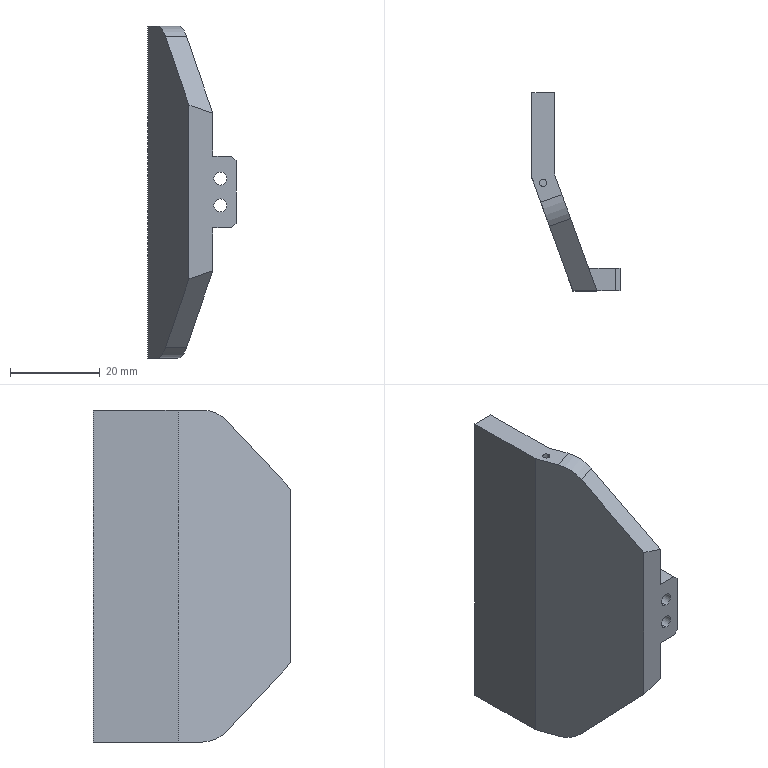NC program | NX | posted with a generic post | part box 19.643 x 44.061 x 74 mm
Lines 1 to 613 of 4832:
N10 G17 G21 G94 G90
(FLOOR_FACING_3 , TOOL : D8开粗)
N12 T02 M6
N14 G54
N16 G17 G0 G90 X44. Y-28.322 B0. C0. S4500 M3
N18 G43 Z29.368 H2
N20 Z2.468
N22 G94 G1 Z-0.532 F800.
N24 X41.
N26 X-41.
N28 Y-24.528
N30 G2 X-40.894 Y-22.939 R12.
N32 G1 X40.894
N34 G3 X38.767 Y-17.557 R12.
N36 G1 X-38.767
N38 G2 X-37.485 Y-16.043 R12.
N40 G1 X-33.616 Y-12.174
N42 X33.616
N44 X28.234 Y-6.792
N46 X-28.234
N48 X-32.477
N50 Z2.468
N52 G0 Z29.368
N54 M5
(FLOOR_FACING_3_COPY , TOOL : D8精光)
N56 T03 M6
N58 G54
N60 G17 G0 G90 X44. Y-28.322 B0. C0. S4500 M3
N62 G43 Z29.368 H3
N64 Z2.368
N66 G94 G1 Z-0.632 F800.
N68 X41.
N70 X-41.
N72 Y-24.528
N74 G2 X-40.894 Y-22.939 R12.
N76 G1 X40.894
N78 G3 X38.767 Y-17.557 R12.
N80 G1 X-38.767
N82 G2 X-37.485 Y-16.043 R12.
N84 G1 X-33.616 Y-12.174
N86 X33.616
N88 X28.234 Y-6.792
N90 X-28.234
N92 X-32.477
N94 Z2.368
N96 G0 Z29.368
N98 M5
(PLANAR_MILL , TOOL : D8开粗)
N100 T02 M6
N102 G54
N104 G17 G0 G90 X-24.188 Y-22.828 B0. C0. S4500 M3
N106 G43 Z29.368 H2
N108 Z0.368
N110 G94 G1 X-26.722 Y-25.362 Z0.363 F2000.
N112 X-26.8 Y-25.55 Z0.362
N114 Y-43.344 Z0.338
N116 X26.8 Z0.263
N118 Y-25.55 Z0.238
N120 X26.722 Y-25.362
N122 X12.775 Y-11.414 Z0.21
N124 X12.481 Y-11.293
N126 X-12.481 Z0.175
N128 X-12.775 Y-11.414 Z0.174
N130 X-26.722 Y-25.362 Z0.147
N132 X-26.8 Y-25.55
N134 Y-43.344 Z0.122
N136 X26.8 Z0.047
N138 Y-25.55 Z0.022
N140 X26.722 Y-25.362
N142 X12.775 Y-11.414 Z-0.006
N144 X12.481 Y-11.293
N146 X-12.481 Z-0.041
N148 X-12.775 Y-11.414 Z-0.042
N150 X-26.722 Y-25.362 Z-0.069
N152 X-26.8 Y-25.55
N154 Y-43.344 Z-0.094
N156 X26.8 Z-0.169
N158 Y-25.55 Z-0.194
N160 X26.722 Y-25.362
N162 X12.775 Y-11.414 Z-0.222
N164 X12.481 Y-11.293
N166 X-12.481 Z-0.257
N168 X-12.775 Y-11.414
N170 X-26.722 Y-25.362 Z-0.285
N172 X-26.8 Y-25.55
N174 Y-43.344 Z-0.31
N176 X26.8 Z-0.385
N178 Y-25.55 Z-0.41
N180 X26.722 Y-25.362
N182 X12.775 Y-11.414 Z-0.438
N184 X12.481 Y-11.293
N186 X-12.481 Z-0.473
N188 X-12.775 Y-11.414
N190 X-26.722 Y-25.362 Z-0.501
N192 X-26.8 Y-25.55
N194 Y-43.344 Z-0.526
N196 X26.8 Z-0.601
N198 Y-25.55 Z-0.626
N200 X26.722 Y-25.362
N202 X12.775 Y-11.414 Z-0.654
N204 X12.481 Y-11.293
N206 X-12.481 Z-0.689
N208 X-12.775 Y-11.414
N210 X-26.722 Y-25.362 Z-0.717
N212 X-26.8 Y-25.55
N214 Y-43.344 Z-0.742
N216 X26.8 Z-0.817
N218 Y-25.55 Z-0.842
N220 X26.722 Y-25.362
N222 X12.775 Y-11.414 Z-0.87
N224 X12.481 Y-11.293
N226 X-12.481 Z-0.905
N228 X-12.775 Y-11.414
N230 X-26.722 Y-25.362 Z-0.933
N232 X-26.8 Y-25.55
N234 Y-43.344 Z-0.958
N236 X26.8 Z-1.033
N238 Y-25.55 Z-1.058
N240 X26.722 Y-25.362
N242 X12.775 Y-11.414 Z-1.085
N244 X12.481 Y-11.293 Z-1.086
N246 X-12.481 Z-1.121
N248 X-12.775 Y-11.414
N250 X-26.722 Y-25.362 Z-1.149
N252 X-26.8 Y-25.55
N254 Y-43.344 Z-1.174
N256 X26.8 Z-1.249
N258 Y-25.55 Z-1.274
N260 X26.722 Y-25.362
N262 X12.775 Y-11.414 Z-1.301
N264 X12.481 Y-11.293 Z-1.302
N266 X-12.481 Z-1.337
N268 X-12.775 Y-11.414
N270 X-26.722 Y-25.362 Z-1.365
N272 X-26.8 Y-25.55
N274 Y-43.344 Z-1.39
N276 X26.8 Z-1.465
N278 Y-25.55 Z-1.489
N280 X26.722 Y-25.362 Z-1.49
N282 X12.775 Y-11.414 Z-1.517
N284 X12.481 Y-11.293 Z-1.518
N286 X-12.481 Z-1.553
N288 X-12.775 Y-11.414
N290 X-26.722 Y-25.362 Z-1.581
N292 X-26.8 Y-25.55
N294 Y-43.344 Z-1.606
N296 X26.8 Z-1.681
N298 Y-25.55 Z-1.705
N300 X26.722 Y-25.362 Z-1.706
N302 X12.775 Y-11.414 Z-1.733
N304 X12.481 Y-11.293 Z-1.734
N306 X-12.481 Z-1.768
N308 X-12.775 Y-11.414 Z-1.769
N310 X-26.722 Y-25.362 Z-1.796
N312 X-26.8 Y-25.55 Z-1.797
N314 Y-43.344 Z-1.822
N316 X26.8 Z-1.896
N318 Y-25.55 Z-1.921
N320 X26.722 Y-25.362 Z-1.922
N322 X12.775 Y-11.414 Z-1.949
N324 X12.481 Y-11.293 Z-1.95
N326 X-12.481 Z-1.984
N328 X-12.775 Y-11.414 Z-1.985
N330 X-26.722 Y-25.362 Z-2.012
N332 X-26.8 Y-25.55 Z-2.013
N334 Y-43.344 Z-2.038
N336 X26.8 Z-2.112
N338 Y-25.55 Z-2.137
N340 X26.722 Y-25.362 Z-2.138
N342 X12.775 Y-11.414 Z-2.165
N344 X12.481 Y-11.293
N346 X-12.481 Z-2.2
N348 X-12.775 Y-11.414 Z-2.201
N350 X-26.722 Y-25.362 Z-2.228
N352 X-26.8 Y-25.55 Z-2.229
N354 Y-43.344 Z-2.253
N356 X26.8 Z-2.328
N358 Y-25.55 Z-2.353
N360 X26.722 Y-25.362
N362 X12.775 Y-11.414 Z-2.381
N364 X12.481 Y-11.293
N366 X-12.481 Z-2.416
N368 X-12.775 Y-11.414 Z-2.417
N370 X-26.722 Y-25.362 Z-2.444
N372 X-26.8 Y-25.55 Z-2.445
N374 Y-43.344 Z-2.469
N376 X26.8 Z-2.544
N378 Y-25.55 Z-2.569
N380 X26.722 Y-25.362
N382 X12.775 Y-11.414 Z-2.597
N384 X12.481 Y-11.293
N386 X-12.481 Z-2.632
N388 X-12.775 Y-11.414 Z-2.633
N390 X-26.722 Y-25.362 Z-2.66
N392 X-26.8 Y-25.55
N394 Y-43.344 Z-2.685
N396 X26.8 Z-2.76
N398 Y-25.55 Z-2.785
N400 X26.722 Y-25.362
N402 X12.775 Y-11.414 Z-2.813
N404 X12.481 Y-11.293
N406 X-12.481 Z-2.848
N408 X-12.775 Y-11.414 Z-2.849
N410 X-26.722 Y-25.362 Z-2.876
N412 X-26.8 Y-25.55
N414 Y-43.344 Z-2.901
N416 X26.8 Z-2.976
N418 Y-25.55 Z-3.001
N420 X26.722 Y-25.362
N422 X12.775 Y-11.414 Z-3.029
N424 X12.481 Y-11.293
N426 X-12.481 Z-3.064
N428 X-12.775 Y-11.414
N430 X-26.722 Y-25.362 Z-3.092
N432 X-26.8 Y-25.55
N434 Y-43.344 Z-3.117
N436 X26.8 Z-3.192
N438 Y-25.55 Z-3.217
N440 X26.722 Y-25.362
N442 X12.775 Y-11.414 Z-3.245
N444 X12.481 Y-11.293
N446 X-12.481 Z-3.28
N448 X-12.775 Y-11.414
N450 X-26.722 Y-25.362 Z-3.308
N452 X-26.8 Y-25.55
N454 Y-43.344 Z-3.333
N456 X26.8 Z-3.408
N458 Y-25.55 Z-3.433
N460 X26.722 Y-25.362
N462 X12.775 Y-11.414 Z-3.461
N464 X12.481 Y-11.293
N466 X-12.481 Z-3.496
N468 X-12.775 Y-11.414
N470 X-26.722 Y-25.362 Z-3.524
N472 X-26.8 Y-25.55
N474 Y-43.344 Z-3.549
N476 X26.8 Z-3.624
N478 Y-25.55 Z-3.649
N480 X26.722 Y-25.362
N482 X12.775 Y-11.414 Z-3.677
N484 X12.481 Y-11.293
N486 X-12.481 Z-3.712
N488 X-12.775 Y-11.414
N490 X-26.722 Y-25.362 Z-3.74
N492 X-26.8 Y-25.55
N494 Y-43.344 Z-3.765
N496 X26.8 Z-3.84
N498 Y-25.55 Z-3.865
N500 X26.722 Y-25.362
N502 X12.775 Y-11.414 Z-3.892
N504 X12.481 Y-11.293 Z-3.893
N506 X-12.481 Z-3.928
N508 X-12.775 Y-11.414
N510 X-26.722 Y-25.362 Z-3.956
N512 X-26.8 Y-25.55
N514 Y-43.344 Z-3.981
N516 X26.8 Z-4.056
N518 Y-25.55 Z-4.081
N520 X26.722 Y-25.362
N522 X12.775 Y-11.414 Z-4.108
N524 X12.481 Y-11.293 Z-4.109
N526 X-12.481 Z-4.144
N528 X-12.775 Y-11.414
N530 X-26.722 Y-25.362 Z-4.172
N532 X-26.8 Y-25.55
N534 Y-43.344 Z-4.197
N536 X26.8 Z-4.272
N538 Y-25.55 Z-4.296
N540 X26.722 Y-25.362 Z-4.297
N542 X12.775 Y-11.414 Z-4.324
N544 X12.481 Y-11.293 Z-4.325
N546 X-12.481 Z-4.36
N548 X-12.775 Y-11.414
N550 X-26.722 Y-25.362 Z-4.388
N552 X-26.8 Y-25.55
N554 Y-43.344 Z-4.413
N556 X26.8 Z-4.488
N558 Y-25.55 Z-4.512
N560 X26.722 Y-25.362 Z-4.513
N562 X12.775 Y-11.414 Z-4.54
N564 X12.481 Y-11.293 Z-4.541
N566 X-12.481 Z-4.575
N568 X-12.775 Y-11.414 Z-4.576
N570 X-26.722 Y-25.362 Z-4.603
N572 X-26.8 Y-25.55 Z-4.604
N574 Y-43.344 Z-4.629
N576 X26.8 Z-4.703
N578 Y-25.55 Z-4.728
N580 X26.722 Y-25.362 Z-4.729
N582 X12.775 Y-11.414 Z-4.756
N584 X12.481 Y-11.293 Z-4.757
N586 X-12.481 Z-4.791
N588 X-12.775 Y-11.414 Z-4.792
N590 X-26.722 Y-25.362 Z-4.819
N592 X-26.8 Y-25.55 Z-4.82
N594 Y-43.344 Z-4.845
N596 X26.8 Z-4.919
N598 Y-25.55 Z-4.944
N600 X26.722 Y-25.362 Z-4.945
N602 X12.775 Y-11.414 Z-4.972
N604 X12.481 Y-11.293
N606 X-12.481 Z-5.007
N608 X-12.775 Y-11.414 Z-5.008
N610 X-26.722 Y-25.362 Z-5.035
N612 X-26.8 Y-25.55 Z-5.036
N614 Y-43.344 Z-5.06
N616 X26.8 Z-5.135
N618 Y-25.55 Z-5.16
N620 X26.722 Y-25.362
N622 X12.775 Y-11.414 Z-5.188
N624 X12.481 Y-11.293
N626 X-12.481 Z-5.223
N628 X-12.775 Y-11.414 Z-5.224
N630 X-26.722 Y-25.362 Z-5.251
N632 X-26.8 Y-25.55 Z-5.252
N634 Y-43.344 Z-5.276
N636 X26.8 Z-5.351
N638 Y-25.55 Z-5.376
N640 X26.722 Y-25.362
N642 X12.775 Y-11.414 Z-5.404
N644 X12.481 Y-11.293
N646 X-12.481 Z-5.439
N648 X-12.775 Y-11.414 Z-5.44
N650 X-26.722 Y-25.362 Z-5.467
N652 X-26.8 Y-25.55
N654 Y-43.344 Z-5.492
N656 X26.8 Z-5.567
N658 Y-25.55 Z-5.592
N660 X26.722 Y-25.362
N662 X12.775 Y-11.414 Z-5.62
N664 X12.481 Y-11.293
N666 X-12.481 Z-5.655
N668 X-12.775 Y-11.414 Z-5.656
N670 X-26.722 Y-25.362 Z-5.683
N672 X-26.8 Y-25.55
N674 Y-43.344 Z-5.708
N676 X26.8 Z-5.783
N678 Y-25.55 Z-5.808
N680 X26.722 Y-25.362
N682 X12.775 Y-11.414 Z-5.836
N684 X12.481 Y-11.293
N686 X-12.481 Z-5.871
N688 X-12.775 Y-11.414
N690 X-26.722 Y-25.362 Z-5.899
N692 X-26.8 Y-25.55
N694 Y-43.344 Z-5.924
N696 X26.8 Z-5.999
N698 Y-25.55 Z-6.024
N700 X26.722 Y-25.362
N702 X12.775 Y-11.414 Z-6.052
N704 X12.481 Y-11.293
N706 X-12.481 Z-6.087
N708 X-12.775 Y-11.414
N710 X-26.722 Y-25.362 Z-6.115
N712 X-26.8 Y-25.55
N714 Y-43.344 Z-6.14
N716 X26.8 Z-6.215
N718 Y-25.55 Z-6.24
N720 X26.722 Y-25.362
N722 X12.775 Y-11.414 Z-6.268
N724 X12.481 Y-11.293
N726 X-12.481 Z-6.303
N728 X-12.775 Y-11.414
N730 X-26.722 Y-25.362 Z-6.331
N732 X-26.8 Y-25.55
N734 Y-43.344 Z-6.356
N736 X26.8 Z-6.431
N738 Y-25.55 Z-6.456
N740 X26.722 Y-25.362
N742 X12.775 Y-11.414 Z-6.484
N744 X12.481 Y-11.293
N746 X-12.481 Z-6.519
N748 X-12.775 Y-11.414
N750 X-26.722 Y-25.362 Z-6.547
N752 X-26.8 Y-25.55
N754 Y-43.344 Z-6.572
N756 X26.8 Z-6.647
N758 Y-25.55 Z-6.672
N760 X26.722 Y-25.362
N762 X12.775 Y-11.414 Z-6.699
N764 X12.481 Y-11.293 Z-6.7
N766 X-12.481 Z-6.735
N768 X-12.775 Y-11.414
N770 X-26.722 Y-25.362 Z-6.763
N772 X-26.8 Y-25.55
N774 Y-43.344 Z-6.788
N776 X26.8 Z-6.863
N778 Y-25.55 Z-6.888
N780 X26.722 Y-25.362
N782 X12.775 Y-11.414 Z-6.915
N784 X12.481 Y-11.293 Z-6.916
N786 X-12.481 Z-6.951
N788 X-12.775 Y-11.414
N790 X-26.722 Y-25.362 Z-6.979
N792 X-26.8 Y-25.55
N794 Y-43.344 Z-7.004
N796 X26.8 Z-7.079
N798 Y-25.55 Z-7.103
N800 X26.722 Y-25.362 Z-7.104
N802 X12.775 Y-11.414 Z-7.131
N804 X12.481 Y-11.293 Z-7.132
N806 X-12.481 Z-7.167
N808 X-12.775 Y-11.414
N810 X-26.722 Y-25.362 Z-7.195
N812 X-26.8 Y-25.55
N814 Y-43.344 Z-7.22
N816 X26.8 Z-7.295
N818 Y-25.55 Z-7.319
N820 X26.722 Y-25.362 Z-7.32
N822 X12.775 Y-11.414 Z-7.347
N824 X12.481 Y-11.293 Z-7.348
N826 X-12.481 Z-7.382
N828 X-12.775 Y-11.414 Z-7.383
N830 X-26.722 Y-25.362 Z-7.41
N832 X-26.8 Y-25.55 Z-7.411
N834 Y-43.344 Z-7.436
N836 X26.8 Z-7.51
N838 Y-25.55 Z-7.535
N840 X26.722 Y-25.362 Z-7.536
N842 X12.775 Y-11.414 Z-7.563
N844 X12.481 Y-11.293 Z-7.564
N846 X-12.481 Z-7.598
N848 X-12.775 Y-11.414 Z-7.599
N850 X-26.722 Y-25.362 Z-7.626
N852 X-26.8 Y-25.55 Z-7.627
N854 Y-43.344 Z-7.652
N856 X26.8 Z-7.726
N858 Y-25.55 Z-7.751
N860 X26.722 Y-25.362
N862 X12.775 Y-11.414 Z-7.779
N864 X12.481 Y-11.293
N866 X-12.481 Z-7.814
N868 X-12.775 Y-11.414 Z-7.815
N870 X-26.722 Y-25.362 Z-7.842
N872 X-26.8 Y-25.55 Z-7.843
N874 Y-43.344 Z-7.867
N876 X26.8 Z-7.942
N878 Y-25.55 Z-7.967
N880 X26.722 Y-25.362
N882 X12.775 Y-11.414 Z-7.995
N884 X12.481 Y-11.293
N886 X-12.481 Z-8.03
N888 X-12.775 Y-11.414 Z-8.031
N890 X-26.722 Y-25.362 Z-8.058
N892 X-26.8 Y-25.55 Z-8.059
N894 Y-43.344 Z-8.083
N896 X26.8 Z-8.158
N898 Y-25.55 Z-8.183
N900 X26.722 Y-25.362
N902 X12.775 Y-11.414 Z-8.211
N904 X12.481 Y-11.293
N906 X-12.481 Z-8.246
N908 X-12.775 Y-11.414 Z-8.247
N910 X-26.722 Y-25.362 Z-8.274
N912 X-26.8 Y-25.55
N914 Y-43.344 Z-8.299
N916 X26.8 Z-8.374
N918 Y-25.55 Z-8.399
N920 X26.722 Y-25.362
N922 X12.775 Y-11.414 Z-8.427
N924 X12.481 Y-11.293
N926 X-12.481 Z-8.462
N928 X-12.775 Y-11.414 Z-8.463
N930 X-26.722 Y-25.362 Z-8.49
N932 X-26.8 Y-25.55
N934 Y-43.344 Z-8.515
N936 X26.8 Z-8.59
N938 Y-25.55 Z-8.615
N940 X26.722 Y-25.362
N942 X12.775 Y-11.414 Z-8.643
N944 X12.481 Y-11.293
N946 X-12.481 Z-8.678
N948 X-12.775 Y-11.414
N950 X-26.722 Y-25.362 Z-8.706
N952 X-26.8 Y-25.55
N954 Y-43.344 Z-8.731
N956 X26.8 Z-8.806
N958 Y-25.55 Z-8.831
N960 X26.722 Y-25.362
N962 X12.775 Y-11.414 Z-8.859
N964 X12.481 Y-11.293
N966 X-12.481 Z-8.894
N968 X-12.775 Y-11.414
N970 X-26.722 Y-25.362 Z-8.922
N972 X-26.8 Y-25.55
N974 Y-43.344 Z-8.947
N976 X26.8 Z-9.022
N978 Y-25.55 Z-9.047
N980 X26.722 Y-25.362
N982 X12.775 Y-11.414 Z-9.075
N984 X12.481 Y-11.293
N986 X-12.481 Z-9.11
N988 X-12.775 Y-11.414
N990 X-26.722 Y-25.362 Z-9.138
N992 X-26.8 Y-25.55
N994 Y-43.344 Z-9.163
N996 X26.8 Z-9.238
N998 Y-25.55 Z-9.263
N1000 X26.722 Y-25.362
N1002 X12.775 Y-11.414 Z-9.29
N1004 X12.481 Y-11.293 Z-9.291
N1006 X-12.481 Z-9.326
N1008 X-12.775 Y-11.414
N1010 X-26.722 Y-25.362 Z-9.354
N1012 X-26.8 Y-25.55
N1014 Y-43.344 Z-9.379
N1016 X26.8 Z-9.454
N1018 Y-25.55 Z-9.479
N1020 X26.722 Y-25.362
N1022 X12.775 Y-11.414 Z-9.506
N1024 X12.481 Y-11.293 Z-9.507
N1026 X-12.481 Z-9.542
N1028 X-12.775 Y-11.414
N1030 X-26.722 Y-25.362 Z-9.57
N1032 X-26.8 Y-25.55
N1034 Y-43.344 Z-9.595
N1036 X0. Z-9.632
N1038 X26.8
N1040 Y-25.771
N1042 G3 X26.566 Y-25.205 R0.8
N1044 G1 X12.887 Y-11.527
N1046 G3 X12.322 Y-11.293 R0.8
N1048 G1 X-12.322
N1050 G3 X-12.887 Y-11.527 R0.8
N1052 G1 X-26.566 Y-25.205
N1054 G3 X-26.8 Y-25.771 R0.8
N1056 G1 Y-43.344
N1058 X0.
N1060 Z-8.632
N1062 G0 Z29.368
N1064 M5
(PLANAR_MILL_COPY , TOOL : D8精光)
N1066 T03 M6
N1068 G54
N1070 G17 G0 G90 X-2. Y-41.456 B0. C0. S4500 M3
N1072 G43 Z29.368 H3
N1074 Z-7.632
N1076 G94 G1 Z-9.632 F600.
N1078 G3 X0. Y-43.456 R2.
N1080 G1 X26.912
N1082 Y-25.771
N1084 G3 X26.645 Y-25.126 R0.912
N1086 G1 X12.966 Y-11.448
N1088 G3 X12.322 Y-11.181 R0.912
N1090 G1 X-12.322
N1092 G3 X-12.966 Y-11.448 R0.912
N1094 G1 X-26.645 Y-25.126
N1096 G3 X-26.912 Y-25.771 R0.912
N1098 G1 Y-43.456
N1100 X0.
N1102 G3 X2. Y-41.456 R2.
N1104 G1 X-2. Y-41.464
N1106 G3 X0. Y-43.464 R2.
N1108 G1 X26.92
N1110 Y-25.771
N1112 G3 X26.651 Y-25.121 R0.92
N1114 G1 X12.972 Y-11.442
N1116 G3 X12.322 Y-11.173 R0.92
N1118 G1 X-12.322
N1120 G3 X-12.972 Y-11.442 R0.92
N1122 G1 X-26.651 Y-25.121
N1124 G3 X-26.92 Y-25.771 R0.92
N1126 G1 Y-43.464
N1128 X0.
N1130 G3 X2. Y-41.464 R2.
N1132 G1 Z-7.632
N1134 G0 Z29.368
(PLANAR_MILL_COPY_COPY , TOOL : D8精光)
N1136 X-2. Y-41.494
N1138 Z-7.632
N1140 G1 Z-9.632
N1142 G3 X0. Y-43.494 R2.
N1144 G1 X26.95
N1146 Y-25.771
N1148 G3 X26.672 Y-25.099 R0.95
N1150 G1 X12.993 Y-11.421
N1152 G3 X12.322 Y-11.143 R0.95
N1154 G1 X-12.322
N1156 G3 X-12.993 Y-11.421 R0.95
N1158 G1 X-26.672 Y-25.099
N1160 G3 X-26.95 Y-25.771 R0.95
N1162 G1 Y-43.494
N1164 X0.
N1166 G3 X2. Y-41.494 R2.
N1168 G1 X-2.
N1170 G3 X0. Y-43.494 R2.
N1172 G1 X26.95
N1174 Y-25.771
N1176 G3 X26.672 Y-25.099 R0.95
N1178 G1 X12.993 Y-11.421
N1180 G3 X12.322 Y-11.143 R0.95
N1182 G1 X-12.322
N1184 G3 X-12.993 Y-11.421 R0.95
N1186 G1 X-26.672 Y-25.099
N1188 G3 X-26.95 Y-25.771 R0.95
N1190 G1 Y-43.494
N1192 X0.
N1194 G3 X2. Y-41.494 R2.
N1196 G1 Z-7.632
N1198 G0 Z29.368
N1200 M5